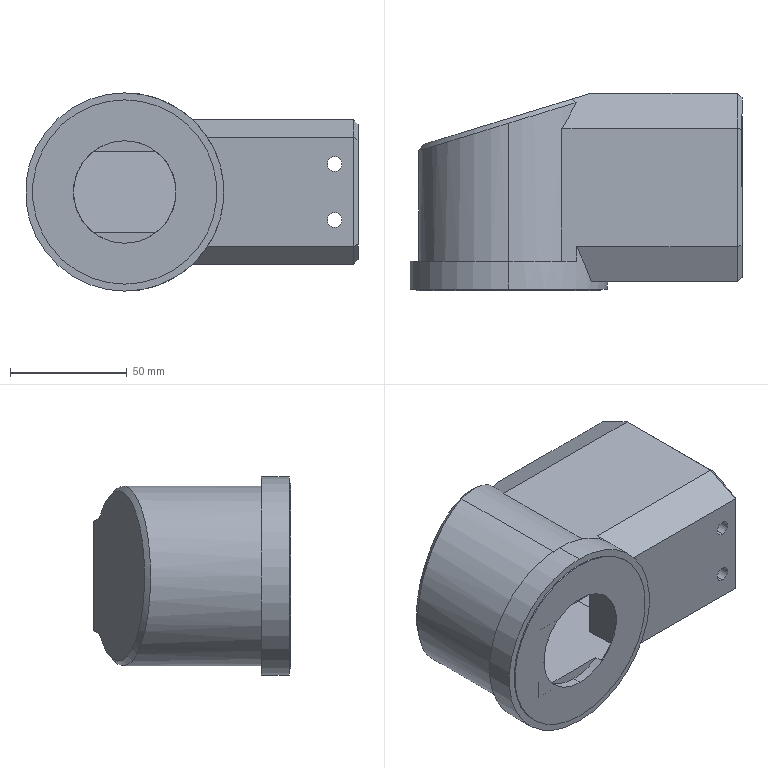Part | SolidWorks | features BaseBody 1 | 1 solid | 63 faces | box 142.5 x 84.5 x 85 mm | volume 382964 mm3 | plane 41 | cylinder 21 | spline 1 | commonest cylinder face diameters 6.2 x12 77 x3 44 x2 79 x2 85 x2